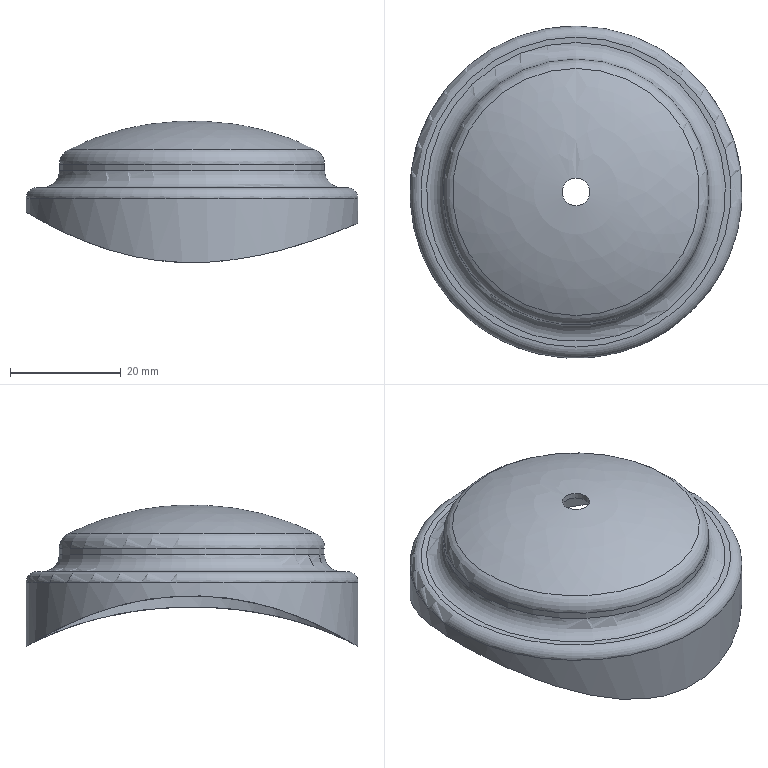Part | STEP file | 1-15 | 1 solid | 16 faces | box 60.001 x 60 x 25.516 mm | volume 4981 mm3 | torus 6 | cylinder 5 | spline 3 | plane 2 | commonest cylinder face diameters 5 x1 46 x1 48 x1 58 x1 60 x1